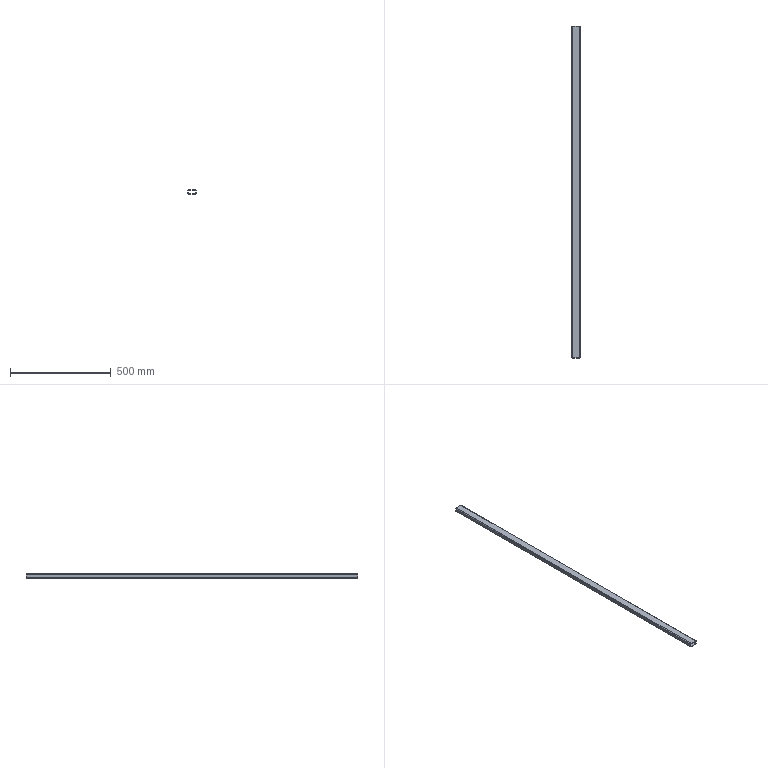Part | SolidWorks | features Extrusion 1 | 1 solid | 18 faces | box 40 x 1650 x 20 mm | volume 352604 mm3 | plane 10 | cylinder 8 | commonest cylinder face diameters 4 x4 8 x4
STEP:
#1=CARTESIAN_POINT('',(-20.,1650.,6.));
#2=VERTEX_POINT('',#1);
#3=CARTESIAN_POINT('',(-16.,1650.,10.));
#4=VERTEX_POINT('',#3);
#5=CARTESIAN_POINT('',(-16.,1650.,6.));
#6=DIRECTION('',(0.,1.,0.));
#7=DIRECTION('',(0.,0.,-1.));
#8=AXIS2_PLACEMENT_3D('',#5,#6,#7);
#9=CIRCLE('',#8,4.);
#10=EDGE_CURVE('',#2,#4,#9,.T.);
#11=ORIENTED_EDGE('',*,*,#10,.T.);
#12=CARTESIAN_POINT('',(16.,1650.,10.));
#13=VERTEX_POINT('',#12);
#14=CARTESIAN_POINT('',(-16.,1650.,10.));
#15=DIRECTION('',(1.,0.,0.));
#16=VECTOR('',#15,1000.);
#17=LINE('',#14,#16);
#18=EDGE_CURVE('',#4,#13,#17,.T.);
#19=ORIENTED_EDGE('',*,*,#18,.T.);
#20=CARTESIAN_POINT('',(20.,1650.,6.));
#21=VERTEX_POINT('',#20);
#22=CARTESIAN_POINT('',(16.,1650.,6.));
#23=DIRECTION('',(0.,1.,0.));
#24=DIRECTION('',(0.,0.,1.));
#25=AXIS2_PLACEMENT_3D('',#22,#23,#24);
#26=CIRCLE('',#25,4.);
#27=EDGE_CURVE('',#13,#21,#26,.T.);
#28=ORIENTED_EDGE('',*,*,#27,.T.);
#29=CARTESIAN_POINT('',(20.,1650.,-6.));
#30=VERTEX_POINT('',#29);
#31=CARTESIAN_POINT('',(20.,1650.,6.));
#32=DIRECTION('',(0.,0.,-1.));
#33=VECTOR('',#32,1000.);
#34=LINE('',#31,#33);
#35=EDGE_CURVE('',#21,#30,#34,.T.);
#36=ORIENTED_EDGE('',*,*,#35,.T.);
#37=CARTESIAN_POINT('',(16.,1650.,-10.));
#38=VERTEX_POINT('',#37);
#39=CARTESIAN_POINT('',(16.,1650.,-6.));
#40=DIRECTION('',(0.,1.,0.));
#41=DIRECTION('',(0.,0.,-1.));
#42=AXIS2_PLACEMENT_3D('',#39,#40,#41);
#43=CIRCLE('',#42,4.);
#44=EDGE_CURVE('',#30,#38,#43,.T.);
#45=ORIENTED_EDGE('',*,*,#44,.T.);
#46=CARTESIAN_POINT('',(-16.,1650.,-10.));
#47=VERTEX_POINT('',#46);
#48=CARTESIAN_POINT('',(-16.,1650.,-10.));
#49=DIRECTION('',(-1.,0.,0.));
#50=VECTOR('',#49,1000.);
#51=LINE('',#48,#50);
#52=EDGE_CURVE('',#38,#47,#51,.T.);
#53=ORIENTED_EDGE('',*,*,#52,.T.);
#54=CARTESIAN_POINT('',(-20.,1650.,-6.));
#55=VERTEX_POINT('',#54);
#56=CARTESIAN_POINT('',(-16.,1650.,-6.));
#57=DIRECTION('',(0.,1.,0.));
#58=DIRECTION('',(0.,0.,-1.));
#59=AXIS2_PLACEMENT_3D('',#56,#57,#58);
#60=CIRCLE('',#59,4.);
#61=EDGE_CURVE('',#47,#55,#60,.T.);
#62=ORIENTED_EDGE('',*,*,#61,.T.);
#63=CARTESIAN_POINT('',(-20.,1650.,6.));
#64=DIRECTION('',(0.,0.,1.));
#65=VECTOR('',#64,1000.);
#66=LINE('',#63,#65);
#67=EDGE_CURVE('',#55,#2,#66,.T.);
#68=ORIENTED_EDGE('',*,*,#67,.T.);
#69=EDGE_LOOP('',(#11,#19,#28,#36,#45,#53,#62,#68));
#70=FACE_OUTER_BOUND('',#69,.T.);
#71=CARTESIAN_POINT('',(-18.,1650.,6.));
#72=VERTEX_POINT('',#71);
#73=CARTESIAN_POINT('',(-16.,1650.,8.));
#74=VERTEX_POINT('',#73);
#75=CARTESIAN_POINT('',(-16.,1650.,6.));
#76=DIRECTION('',(0.,1.,0.));
#77=DIRECTION('',(0.,0.,-1.));
#78=AXIS2_PLACEMENT_3D('',#75,#76,#77);
#79=CIRCLE('',#78,2.);
#80=EDGE_CURVE('',#72,#74,#79,.T.);
#81=ORIENTED_EDGE('',*,*,#80,.F.);
#82=CARTESIAN_POINT('',(-18.,1650.,-6.));
#83=VERTEX_POINT('',#82);
#84=CARTESIAN_POINT('',(-18.,1650.,6.));
#85=DIRECTION('',(0.,0.,1.));
#86=VECTOR('',#85,1000.);
#87=LINE('',#84,#86);
#88=EDGE_CURVE('',#83,#72,#87,.T.);
#89=ORIENTED_EDGE('',*,*,#88,.F.);
#90=CARTESIAN_POINT('',(-16.,1650.,-8.));
#91=VERTEX_POINT('',#90);
#92=CARTESIAN_POINT('',(-16.,1650.,-6.));
#93=DIRECTION('',(0.,1.,0.));
#94=DIRECTION('',(0.,0.,-1.));
#95=AXIS2_PLACEMENT_3D('',#92,#93,#94);
#96=CIRCLE('',#95,2.);
#97=EDGE_CURVE('',#91,#83,#96,.T.);
#98=ORIENTED_EDGE('',*,*,#97,.F.);
#99=CARTESIAN_POINT('',(16.,1650.,-8.));
#100=VERTEX_POINT('',#99);
#101=CARTESIAN_POINT('',(-16.,1650.,-8.));
#102=DIRECTION('',(-1.,0.,0.));
#103=VECTOR('',#102,1000.);
#104=LINE('',#101,#103);
#105=EDGE_CURVE('',#100,#91,#104,.T.);
#106=ORIENTED_EDGE('',*,*,#105,.F.);
#107=CARTESIAN_POINT('',(18.,1650.,-6.));
#108=VERTEX_POINT('',#107);
#109=CARTESIAN_POINT('',(16.,1650.,-6.));
#110=DIRECTION('',(0.,1.,0.));
#111=DIRECTION('',(0.,0.,-1.));
#112=AXIS2_PLACEMENT_3D('',#109,#110,#111);
#113=CIRCLE('',#112,2.);
#114=EDGE_CURVE('',#108,#100,#113,.T.);
#115=ORIENTED_EDGE('',*,*,#114,.F.);
#116=CARTESIAN_POINT('',(18.,1650.,6.));
#117=VERTEX_POINT('',#116);
#118=CARTESIAN_POINT('',(18.,1650.,6.));
#119=DIRECTION('',(0.,0.,-1.));
#120=VECTOR('',#119,1000.);
#121=LINE('',#118,#120);
#122=EDGE_CURVE('',#117,#108,#121,.T.);
#123=ORIENTED_EDGE('',*,*,#122,.F.);
#124=CARTESIAN_POINT('',(16.,1650.,8.));
#125=VERTEX_POINT('',#124);
#126=CARTESIAN_POINT('',(16.,1650.,6.));
#127=DIRECTION('',(0.,1.,0.));
#128=DIRECTION('',(0.,0.,1.));
#129=AXIS2_PLACEMENT_3D('',#126,#127,#128);
#130=CIRCLE('',#129,2.);
#131=EDGE_CURVE('',#125,#117,#130,.T.);
#132=ORIENTED_EDGE('',*,*,#131,.F.);
#133=CARTESIAN_POINT('',(-16.,1650.,8.));
#134=DIRECTION('',(1.,0.,0.));
#135=VECTOR('',#134,1000.);
#136=LINE('',#133,#135);
#137=EDGE_CURVE('',#74,#125,#136,.T.);
#138=ORIENTED_EDGE('',*,*,#137,.F.);
#139=EDGE_LOOP('',(#81,#89,#98,#106,#115,#123,#132,#138));
#140=FACE_BOUND('',#139,.T.);
#141=CARTESIAN_POINT('',(-16.,1650.,6.));
#142=DIRECTION('',(0.,-1.,0.));
#143=DIRECTION('',(0.,0.,-1.));
#144=AXIS2_PLACEMENT_3D('',#141,#142,#143);
#145=PLANE('',#144);
#146=ADVANCED_FACE('',(#70,#140),#145,.F.);
#147=CARTESIAN_POINT('',(-20.,0.,6.));
#148=VERTEX_POINT('',#147);
#149=CARTESIAN_POINT('',(-16.,0.,10.));
#150=VERTEX_POINT('',#149);
#151=CARTESIAN_POINT('',(-16.,0.,6.));
#152=DIRECTION('',(0.,1.,0.));
#153=DIRECTION('',(0.,0.,-1.));
#154=AXIS2_PLACEMENT_3D('',#151,#152,#153);
#155=CIRCLE('',#154,4.);
#156=EDGE_CURVE('',#148,#150,#155,.T.);
#157=ORIENTED_EDGE('',*,*,#156,.F.);
#158=CARTESIAN_POINT('',(-20.,0.,-6.));
#159=VERTEX_POINT('',#158);
#160=CARTESIAN_POINT('',(-20.,0.,6.));
#161=DIRECTION('',(0.,0.,1.));
#162=VECTOR('',#161,1000.);
#163=LINE('',#160,#162);
#164=EDGE_CURVE('',#159,#148,#163,.T.);
#165=ORIENTED_EDGE('',*,*,#164,.F.);
#166=CARTESIAN_POINT('',(-16.,0.,-10.));
#167=VERTEX_POINT('',#166);
#168=CARTESIAN_POINT('',(-16.,0.,-6.));
#169=DIRECTION('',(0.,1.,0.));
#170=DIRECTION('',(0.,0.,-1.));
#171=AXIS2_PLACEMENT_3D('',#168,#169,#170);
#172=CIRCLE('',#171,4.);
#173=EDGE_CURVE('',#167,#159,#172,.T.);
#174=ORIENTED_EDGE('',*,*,#173,.F.);
#175=CARTESIAN_POINT('',(16.,0.,-10.));
#176=VERTEX_POINT('',#175);
#177=CARTESIAN_POINT('',(-16.,0.,-10.));
#178=DIRECTION('',(-1.,0.,0.));
#179=VECTOR('',#178,1000.);
#180=LINE('',#177,#179);
#181=EDGE_CURVE('',#176,#167,#180,.T.);
#182=ORIENTED_EDGE('',*,*,#181,.F.);
#183=CARTESIAN_POINT('',(20.,0.,-6.));
#184=VERTEX_POINT('',#183);
#185=CARTESIAN_POINT('',(16.,0.,-6.));
#186=DIRECTION('',(0.,1.,0.));
#187=DIRECTION('',(0.,0.,-1.));
#188=AXIS2_PLACEMENT_3D('',#185,#186,#187);
#189=CIRCLE('',#188,4.);
#190=EDGE_CURVE('',#184,#176,#189,.T.);
#191=ORIENTED_EDGE('',*,*,#190,.F.);
#192=CARTESIAN_POINT('',(20.,0.,6.));
#193=VERTEX_POINT('',#192);
#194=CARTESIAN_POINT('',(20.,0.,6.));
#195=DIRECTION('',(0.,0.,-1.));
#196=VECTOR('',#195,1000.);
#197=LINE('',#194,#196);
#198=EDGE_CURVE('',#193,#184,#197,.T.);
#199=ORIENTED_EDGE('',*,*,#198,.F.);
#200=CARTESIAN_POINT('',(16.,0.,10.));
#201=VERTEX_POINT('',#200);
#202=CARTESIAN_POINT('',(16.,0.,6.));
#203=DIRECTION('',(0.,1.,0.));
#204=DIRECTION('',(0.,0.,1.));
#205=AXIS2_PLACEMENT_3D('',#202,#203,#204);
#206=CIRCLE('',#205,4.);
#207=EDGE_CURVE('',#201,#193,#206,.T.);
#208=ORIENTED_EDGE('',*,*,#207,.F.);
#209=CARTESIAN_POINT('',(-16.,0.,10.));
#210=DIRECTION('',(1.,0.,0.));
#211=VECTOR('',#210,1000.);
#212=LINE('',#209,#211);
#213=EDGE_CURVE('',#150,#201,#212,.T.);
#214=ORIENTED_EDGE('',*,*,#213,.F.);
#215=EDGE_LOOP('',(#157,#165,#174,#182,#191,#199,#208,#214));
#216=FACE_OUTER_BOUND('',#215,.T.);
#217=CARTESIAN_POINT('',(-18.,0.,-6.));
#218=VERTEX_POINT('',#217);
#219=CARTESIAN_POINT('',(-18.,0.,6.));
#220=VERTEX_POINT('',#219);
#221=CARTESIAN_POINT('',(-18.,0.,6.));
#222=DIRECTION('',(0.,0.,1.));
#223=VECTOR('',#222,1000.);
#224=LINE('',#221,#223);
#225=EDGE_CURVE('',#218,#220,#224,.T.);
#226=ORIENTED_EDGE('',*,*,#225,.T.);
#227=CARTESIAN_POINT('',(-16.,0.,8.));
#228=VERTEX_POINT('',#227);
#229=CARTESIAN_POINT('',(-16.,0.,6.));
#230=DIRECTION('',(0.,1.,0.));
#231=DIRECTION('',(0.,0.,-1.));
#232=AXIS2_PLACEMENT_3D('',#229,#230,#231);
#233=CIRCLE('',#232,2.);
#234=EDGE_CURVE('',#220,#228,#233,.T.);
#235=ORIENTED_EDGE('',*,*,#234,.T.);
#236=CARTESIAN_POINT('',(16.,0.,8.));
#237=VERTEX_POINT('',#236);
#238=CARTESIAN_POINT('',(-16.,0.,8.));
#239=DIRECTION('',(1.,0.,0.));
#240=VECTOR('',#239,1000.);
#241=LINE('',#238,#240);
#242=EDGE_CURVE('',#228,#237,#241,.T.);
#243=ORIENTED_EDGE('',*,*,#242,.T.);
#244=CARTESIAN_POINT('',(18.,0.,6.));
#245=VERTEX_POINT('',#244);
#246=CARTESIAN_POINT('',(16.,0.,6.));
#247=DIRECTION('',(0.,1.,0.));
#248=DIRECTION('',(0.,0.,1.));
#249=AXIS2_PLACEMENT_3D('',#246,#247,#248);
#250=CIRCLE('',#249,2.);
#251=EDGE_CURVE('',#237,#245,#250,.T.);
#252=ORIENTED_EDGE('',*,*,#251,.T.);
#253=CARTESIAN_POINT('',(18.,0.,-6.));
#254=VERTEX_POINT('',#253);
#255=CARTESIAN_POINT('',(18.,0.,6.));
#256=DIRECTION('',(0.,0.,-1.));
#257=VECTOR('',#256,1000.);
#258=LINE('',#255,#257);
#259=EDGE_CURVE('',#245,#254,#258,.T.);
#260=ORIENTED_EDGE('',*,*,#259,.T.);
#261=CARTESIAN_POINT('',(16.,0.,-8.));
#262=VERTEX_POINT('',#261);
#263=CARTESIAN_POINT('',(16.,0.,-6.));
#264=DIRECTION('',(0.,1.,0.));
#265=DIRECTION('',(0.,0.,-1.));
#266=AXIS2_PLACEMENT_3D('',#263,#264,#265);
#267=CIRCLE('',#266,2.);
#268=EDGE_CURVE('',#254,#262,#267,.T.);
#269=ORIENTED_EDGE('',*,*,#268,.T.);
#270=CARTESIAN_POINT('',(-16.,0.,-8.));
#271=VERTEX_POINT('',#270);
#272=CARTESIAN_POINT('',(-16.,0.,-8.));
#273=DIRECTION('',(-1.,0.,0.));
#274=VECTOR('',#273,1000.);
#275=LINE('',#272,#274);
#276=EDGE_CURVE('',#262,#271,#275,.T.);
#277=ORIENTED_EDGE('',*,*,#276,.T.);
#278=CARTESIAN_POINT('',(-16.,0.,-6.));
#279=DIRECTION('',(0.,1.,0.));
#280=DIRECTION('',(0.,0.,-1.));
#281=AXIS2_PLACEMENT_3D('',#278,#279,#280);
#282=CIRCLE('',#281,2.);
#283=EDGE_CURVE('',#271,#218,#282,.T.);
#284=ORIENTED_EDGE('',*,*,#283,.T.);
#285=EDGE_LOOP('',(#226,#235,#243,#252,#260,#269,#277,#284));
#286=FACE_BOUND('',#285,.T.);
#287=CARTESIAN_POINT('',(-16.,0.,6.));
#288=DIRECTION('',(0.,-1.,0.));
#289=DIRECTION('',(0.,0.,-1.));
#290=AXIS2_PLACEMENT_3D('',#287,#288,#289);
#291=PLANE('',#290);
#292=ADVANCED_FACE('',(#216,#286),#291,.T.);
#293=ORIENTED_EDGE('',*,*,#156,.T.);
#294=CARTESIAN_POINT('',(-16.,1650.,10.));
#295=DIRECTION('',(0.,-1.,0.));
#296=VECTOR('',#295,1000.);
#297=LINE('',#294,#296);
#298=EDGE_CURVE('',#4,#150,#297,.T.);
#299=ORIENTED_EDGE('',*,*,#298,.F.);
#300=ORIENTED_EDGE('',*,*,#10,.F.);
#301=CARTESIAN_POINT('',(-20.,1650.,6.));
#302=DIRECTION('',(0.,-1.,0.));
#303=VECTOR('',#302,1000.);
#304=LINE('',#301,#303);
#305=EDGE_CURVE('',#2,#148,#304,.T.);
#306=ORIENTED_EDGE('',*,*,#305,.T.);
#307=EDGE_LOOP('',(#293,#299,#300,#306));
#308=FACE_OUTER_BOUND('',#307,.T.);
#309=CARTESIAN_POINT('',(-16.,1650.,6.));
#310=DIRECTION('',(0.,-1.,0.));
#311=DIRECTION('',(0.,0.,-1.));
#312=AXIS2_PLACEMENT_3D('',#309,#310,#311);
#313=CYLINDRICAL_SURFACE('',#312,4.);
#314=ADVANCED_FACE('',(#308),#313,.T.);
#315=ORIENTED_EDGE('',*,*,#213,.T.);
#316=CARTESIAN_POINT('',(16.,1650.,10.));
#317=DIRECTION('',(0.,-1.,0.));
#318=VECTOR('',#317,1000.);
#319=LINE('',#316,#318);
#320=EDGE_CURVE('',#13,#201,#319,.T.);
#321=ORIENTED_EDGE('',*,*,#320,.F.);
#322=ORIENTED_EDGE('',*,*,#18,.F.);
#323=ORIENTED_EDGE('',*,*,#298,.T.);
#324=EDGE_LOOP('',(#315,#321,#322,#323));
#325=FACE_OUTER_BOUND('',#324,.T.);
#326=CARTESIAN_POINT('',(-16.,1650.,10.));
#327=DIRECTION('',(0.,0.,-1.));
#328=DIRECTION('',(-1.,0.,0.));
#329=AXIS2_PLACEMENT_3D('',#326,#327,#328);
#330=PLANE('',#329);
#331=ADVANCED_FACE('',(#325),#330,.F.);
#332=ORIENTED_EDGE('',*,*,#207,.T.);
#333=CARTESIAN_POINT('',(20.,1650.,6.));
#334=DIRECTION('',(0.,-1.,0.));
#335=VECTOR('',#334,1000.);
#336=LINE('',#333,#335);
#337=EDGE_CURVE('',#21,#193,#336,.T.);
#338=ORIENTED_EDGE('',*,*,#337,.F.);
#339=ORIENTED_EDGE('',*,*,#27,.F.);
#340=ORIENTED_EDGE('',*,*,#320,.T.);
#341=EDGE_LOOP('',(#332,#338,#339,#340));
#342=FACE_OUTER_BOUND('',#341,.T.);
#343=CARTESIAN_POINT('',(16.,1650.,6.));
#344=DIRECTION('',(0.,-1.,0.));
#345=DIRECTION('',(0.,0.,-1.));
#346=AXIS2_PLACEMENT_3D('',#343,#344,#345);
#347=CYLINDRICAL_SURFACE('',#346,4.);
#348=ADVANCED_FACE('',(#342),#347,.T.);
#349=ORIENTED_EDGE('',*,*,#198,.T.);
#350=CARTESIAN_POINT('',(20.,1650.,-6.));
#351=DIRECTION('',(0.,-1.,0.));
#352=VECTOR('',#351,1000.);
#353=LINE('',#350,#352);
#354=EDGE_CURVE('',#30,#184,#353,.T.);
#355=ORIENTED_EDGE('',*,*,#354,.F.);
#356=ORIENTED_EDGE('',*,*,#35,.F.);
#357=ORIENTED_EDGE('',*,*,#337,.T.);
#358=EDGE_LOOP('',(#349,#355,#356,#357));
#359=FACE_OUTER_BOUND('',#358,.T.);
#360=CARTESIAN_POINT('',(20.,1650.,6.));
#361=DIRECTION('',(-1.,0.,0.));
#362=DIRECTION('',(0.,0.,1.));
#363=AXIS2_PLACEMENT_3D('',#360,#361,#362);
#364=PLANE('',#363);
#365=ADVANCED_FACE('',(#359),#364,.F.);
#366=ORIENTED_EDGE('',*,*,#190,.T.);
#367=CARTESIAN_POINT('',(16.,1650.,-10.));
#368=DIRECTION('',(0.,-1.,0.));
#369=VECTOR('',#368,1000.);
#370=LINE('',#367,#369);
#371=EDGE_CURVE('',#38,#176,#370,.T.);
#372=ORIENTED_EDGE('',*,*,#371,.F.);
#373=ORIENTED_EDGE('',*,*,#44,.F.);
#374=ORIENTED_EDGE('',*,*,#354,.T.);
#375=EDGE_LOOP('',(#366,#372,#373,#374));
#376=FACE_OUTER_BOUND('',#375,.T.);
#377=CARTESIAN_POINT('',(16.,1650.,-6.));
#378=DIRECTION('',(0.,-1.,0.));
#379=DIRECTION('',(0.,0.,-1.));
#380=AXIS2_PLACEMENT_3D('',#377,#378,#379);
#381=CYLINDRICAL_SURFACE('',#380,4.);
#382=ADVANCED_FACE('',(#376),#381,.T.);
#383=ORIENTED_EDGE('',*,*,#181,.T.);
#384=CARTESIAN_POINT('',(-16.,1650.,-10.));
#385=DIRECTION('',(0.,-1.,0.));
#386=VECTOR('',#385,1000.);
#387=LINE('',#384,#386);
#388=EDGE_CURVE('',#47,#167,#387,.T.);
#389=ORIENTED_EDGE('',*,*,#388,.F.);
#390=ORIENTED_EDGE('',*,*,#52,.F.);
#391=ORIENTED_EDGE('',*,*,#371,.T.);
#392=EDGE_LOOP('',(#383,#389,#390,#391));
#393=FACE_OUTER_BOUND('',#392,.T.);
#394=CARTESIAN_POINT('',(-16.,1650.,-10.));
#395=DIRECTION('',(0.,0.,1.));
#396=DIRECTION('',(1.,0.,0.));
#397=AXIS2_PLACEMENT_3D('',#394,#395,#396);
#398=PLANE('',#397);
#399=ADVANCED_FACE('',(#393),#398,.F.);
#400=ORIENTED_EDGE('',*,*,#173,.T.);
#401=CARTESIAN_POINT('',(-20.,1650.,-6.));
#402=DIRECTION('',(0.,-1.,0.));
#403=VECTOR('',#402,1000.);
#404=LINE('',#401,#403);
#405=EDGE_CURVE('',#55,#159,#404,.T.);
#406=ORIENTED_EDGE('',*,*,#405,.F.);
#407=ORIENTED_EDGE('',*,*,#61,.F.);
#408=ORIENTED_EDGE('',*,*,#388,.T.);
#409=EDGE_LOOP('',(#400,#406,#407,#408));
#410=FACE_OUTER_BOUND('',#409,.T.);
#411=CARTESIAN_POINT('',(-16.,1650.,-6.));
#412=DIRECTION('',(0.,-1.,0.));
#413=DIRECTION('',(0.,0.,-1.));
#414=AXIS2_PLACEMENT_3D('',#411,#412,#413);
#415=CYLINDRICAL_SURFACE('',#414,4.);
#416=ADVANCED_FACE('',(#410),#415,.T.);
#417=ORIENTED_EDGE('',*,*,#164,.T.);
#418=ORIENTED_EDGE('',*,*,#305,.F.);
#419=ORIENTED_EDGE('',*,*,#67,.F.);
#420=ORIENTED_EDGE('',*,*,#405,.T.);
#421=EDGE_LOOP('',(#417,#418,#419,#420));
#422=FACE_OUTER_BOUND('',#421,.T.);
#423=CARTESIAN_POINT('',(-20.,1650.,6.));
#424=DIRECTION('',(1.,0.,0.));
#425=DIRECTION('',(0.,0.,-1.));
#426=AXIS2_PLACEMENT_3D('',#423,#424,#425);
#427=PLANE('',#426);
#428=ADVANCED_FACE('',(#422),#427,.F.);
#429=ORIENTED_EDGE('',*,*,#234,.F.);
#430=CARTESIAN_POINT('',(-18.,1650.,6.));
#431=DIRECTION('',(0.,-1.,0.));
#432=VECTOR('',#431,1000.);
#433=LINE('',#430,#432);
#434=EDGE_CURVE('',#72,#220,#433,.T.);
#435=ORIENTED_EDGE('',*,*,#434,.F.);
#436=ORIENTED_EDGE('',*,*,#80,.T.);
#437=CARTESIAN_POINT('',(-16.,1650.,8.));
#438=DIRECTION('',(0.,-1.,0.));
#439=VECTOR('',#438,1000.);
#440=LINE('',#437,#439);
#441=EDGE_CURVE('',#74,#228,#440,.T.);
#442=ORIENTED_EDGE('',*,*,#441,.T.);
#443=EDGE_LOOP('',(#429,#435,#436,#442));
#444=FACE_OUTER_BOUND('',#443,.T.);
#445=CARTESIAN_POINT('',(-16.,1650.,6.));
#446=DIRECTION('',(0.,-1.,0.));
#447=DIRECTION('',(0.,0.,-1.));
#448=AXIS2_PLACEMENT_3D('',#445,#446,#447);
#449=CYLINDRICAL_SURFACE('',#448,2.);
#450=ADVANCED_FACE('',(#444),#449,.F.);
#451=ORIENTED_EDGE('',*,*,#242,.F.);
#452=ORIENTED_EDGE('',*,*,#441,.F.);
#453=ORIENTED_EDGE('',*,*,#137,.T.);
#454=CARTESIAN_POINT('',(16.,1650.,8.));
#455=DIRECTION('',(0.,-1.,0.));
#456=VECTOR('',#455,1000.);
#457=LINE('',#454,#456);
#458=EDGE_CURVE('',#125,#237,#457,.T.);
#459=ORIENTED_EDGE('',*,*,#458,.T.);
#460=EDGE_LOOP('',(#451,#452,#453,#459));
#461=FACE_OUTER_BOUND('',#460,.T.);
#462=CARTESIAN_POINT('',(-16.,1650.,8.));
#463=DIRECTION('',(0.,0.,-1.));
#464=DIRECTION('',(-1.,0.,0.));
#465=AXIS2_PLACEMENT_3D('',#462,#463,#464);
#466=PLANE('',#465);
#467=ADVANCED_FACE('',(#461),#466,.T.);
#468=ORIENTED_EDGE('',*,*,#251,.F.);
#469=ORIENTED_EDGE('',*,*,#458,.F.);
#470=ORIENTED_EDGE('',*,*,#131,.T.);
#471=CARTESIAN_POINT('',(18.,1650.,6.));
#472=DIRECTION('',(0.,-1.,0.));
#473=VECTOR('',#472,1000.);
#474=LINE('',#471,#473);
#475=EDGE_CURVE('',#117,#245,#474,.T.);
#476=ORIENTED_EDGE('',*,*,#475,.T.);
#477=EDGE_LOOP('',(#468,#469,#470,#476));
#478=FACE_OUTER_BOUND('',#477,.T.);
#479=CARTESIAN_POINT('',(16.,1650.,6.));
#480=DIRECTION('',(0.,-1.,0.));
#481=DIRECTION('',(0.,0.,-1.));
#482=AXIS2_PLACEMENT_3D('',#479,#480,#481);
#483=CYLINDRICAL_SURFACE('',#482,2.);
#484=ADVANCED_FACE('',(#478),#483,.F.);
#485=ORIENTED_EDGE('',*,*,#259,.F.);
#486=ORIENTED_EDGE('',*,*,#475,.F.);
#487=ORIENTED_EDGE('',*,*,#122,.T.);
#488=CARTESIAN_POINT('',(18.,1650.,-6.));
#489=DIRECTION('',(0.,-1.,0.));
#490=VECTOR('',#489,1000.);
#491=LINE('',#488,#490);
#492=EDGE_CURVE('',#108,#254,#491,.T.);
#493=ORIENTED_EDGE('',*,*,#492,.T.);
#494=EDGE_LOOP('',(#485,#486,#487,#493));
#495=FACE_OUTER_BOUND('',#494,.T.);
#496=CARTESIAN_POINT('',(18.,1650.,6.));
#497=DIRECTION('',(-1.,0.,0.));
#498=DIRECTION('',(0.,0.,1.));
#499=AXIS2_PLACEMENT_3D('',#496,#497,#498);
#500=PLANE('',#499);
#501=ADVANCED_FACE('',(#495),#500,.T.);
#502=ORIENTED_EDGE('',*,*,#268,.F.);
#503=ORIENTED_EDGE('',*,*,#492,.F.);
#504=ORIENTED_EDGE('',*,*,#114,.T.);
#505=CARTESIAN_POINT('',(16.,1650.,-8.));
#506=DIRECTION('',(0.,-1.,0.));
#507=VECTOR('',#506,1000.);
#508=LINE('',#505,#507);
#509=EDGE_CURVE('',#100,#262,#508,.T.);
#510=ORIENTED_EDGE('',*,*,#509,.T.);
#511=EDGE_LOOP('',(#502,#503,#504,#510));
#512=FACE_OUTER_BOUND('',#511,.T.);
#513=CARTESIAN_POINT('',(16.,1650.,-6.));
#514=DIRECTION('',(0.,-1.,0.));
#515=DIRECTION('',(0.,0.,-1.));
#516=AXIS2_PLACEMENT_3D('',#513,#514,#515);
#517=CYLINDRICAL_SURFACE('',#516,2.);
#518=ADVANCED_FACE('',(#512),#517,.F.);
#519=ORIENTED_EDGE('',*,*,#276,.F.);
#520=ORIENTED_EDGE('',*,*,#509,.F.);
#521=ORIENTED_EDGE('',*,*,#105,.T.);
#522=CARTESIAN_POINT('',(-16.,1650.,-8.));
#523=DIRECTION('',(0.,-1.,0.));
#524=VECTOR('',#523,1000.);
#525=LINE('',#522,#524);
#526=EDGE_CURVE('',#91,#271,#525,.T.);
#527=ORIENTED_EDGE('',*,*,#526,.T.);
#528=EDGE_LOOP('',(#519,#520,#521,#527));
#529=FACE_OUTER_BOUND('',#528,.T.);
#530=CARTESIAN_POINT('',(-16.,1650.,-8.));
#531=DIRECTION('',(0.,0.,1.));
#532=DIRECTION('',(1.,0.,0.));
#533=AXIS2_PLACEMENT_3D('',#530,#531,#532);
#534=PLANE('',#533);
#535=ADVANCED_FACE('',(#529),#534,.T.);
#536=ORIENTED_EDGE('',*,*,#283,.F.);
#537=ORIENTED_EDGE('',*,*,#526,.F.);
#538=ORIENTED_EDGE('',*,*,#97,.T.);
#539=CARTESIAN_POINT('',(-18.,1650.,-6.));
#540=DIRECTION('',(0.,-1.,0.));
#541=VECTOR('',#540,1000.);
#542=LINE('',#539,#541);
#543=EDGE_CURVE('',#83,#218,#542,.T.);
#544=ORIENTED_EDGE('',*,*,#543,.T.);
#545=EDGE_LOOP('',(#536,#537,#538,#544));
#546=FACE_OUTER_BOUND('',#545,.T.);
#547=CARTESIAN_POINT('',(-16.,1650.,-6.));
#548=DIRECTION('',(0.,-1.,0.));
#549=DIRECTION('',(0.,0.,-1.));
#550=AXIS2_PLACEMENT_3D('',#547,#548,#549);
#551=CYLINDRICAL_SURFACE('',#550,2.);
#552=ADVANCED_FACE('',(#546),#551,.F.);
#553=ORIENTED_EDGE('',*,*,#225,.F.);
#554=ORIENTED_EDGE('',*,*,#543,.F.);
#555=ORIENTED_EDGE('',*,*,#88,.T.);
#556=ORIENTED_EDGE('',*,*,#434,.T.);
#557=EDGE_LOOP('',(#553,#554,#555,#556));
#558=FACE_OUTER_BOUND('',#557,.T.);
#559=CARTESIAN_POINT('',(-18.,1650.,6.));
#560=DIRECTION('',(1.,0.,0.));
#561=DIRECTION('',(0.,0.,-1.));
#562=AXIS2_PLACEMENT_3D('',#559,#560,#561);
#563=PLANE('',#562);
#564=ADVANCED_FACE('',(#558),#563,.T.);
#565=CLOSED_SHELL('',(#146,#292,#314,#331,#348,#365,#382,#399,#416,#428,#450,#467,#484,#501,#518,#535,#552,#564));
#566=MANIFOLD_SOLID_BREP('',#565);
#567=CARTESIAN_POINT('',(0.,0.,0.));
#568=DIRECTION('',(0.,0.,1.));
#569=DIRECTION('',(1.,0.,0.));
#570=AXIS2_PLACEMENT_3D('',#567,#568,#569);
#571=(LENGTH_UNIT()NAMED_UNIT(*)SI_UNIT(.MILLI.,.METRE.));
#572=UNCERTAINTY_MEASURE_WITH_UNIT(LENGTH_MEASURE(0.00001),#571,'','');
#573=(NAMED_UNIT(*)PLANE_ANGLE_UNIT()SI_UNIT($,.RADIAN.));
#574=(NAMED_UNIT(*)SI_UNIT($,.STERADIAN.)SOLID_ANGLE_UNIT());
#575=(GEOMETRIC_REPRESENTATION_CONTEXT(3)GLOBAL_UNCERTAINTY_ASSIGNED_CONTEXT((#572))GLOBAL_UNIT_ASSIGNED_CONTEXT((#571,#573,#574))REPRESENTATION_CONTEXT('',''));
#576=ADVANCED_BREP_SHAPE_REPRESENTATION('',(#566,#570),#575);